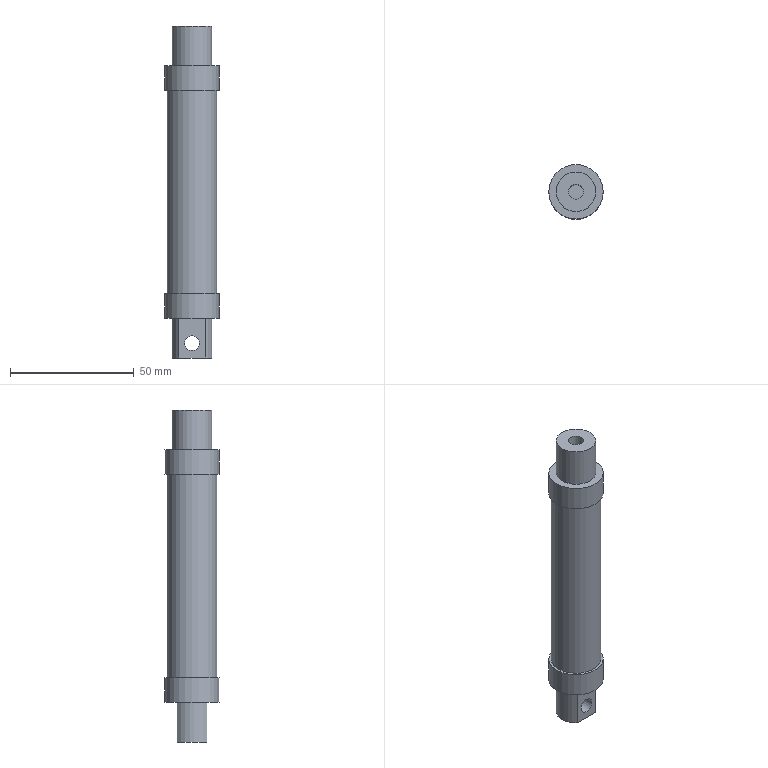Part | NX | features BREP 1, DATUM_CSYS 1 | 1 solid | 17 faces | box 22 x 22 x 134 mm | volume 36167 mm3 | plane 9 | cylinder 8 | commonest cylinder face diameters 16 x3 6 x2 22 x2 20 x1
STEP:
#1=CARTESIAN_POINT('',(11.,0.,92.));
#2=VERTEX_POINT('',#1);
#3=CARTESIAN_POINT('',(0.,0.,92.));
#4=DIRECTION('',(0.,0.,1.));
#5=DIRECTION('',(1.,0.,0.));
#6=AXIS2_PLACEMENT_3D('',#3,#4,#5);
#7=CIRCLE('',#6,11.);
#8=EDGE_CURVE('',#2,#2,#7,.T.);
#9=ORIENTED_EDGE('',*,*,#8,.T.);
#10=EDGE_LOOP('',(#9));
#11=FACE_BOUND('',#10,.T.);
#12=CARTESIAN_POINT('',(8.,0.,92.));
#13=VERTEX_POINT('',#12);
#14=CARTESIAN_POINT('',(0.,0.,92.));
#15=DIRECTION('',(0.,0.,1.));
#16=DIRECTION('',(1.,0.,0.));
#17=AXIS2_PLACEMENT_3D('',#14,#15,#16);
#18=CIRCLE('',#17,8.);
#19=EDGE_CURVE('',#13,#13,#18,.T.);
#20=ORIENTED_EDGE('',*,*,#19,.F.);
#21=EDGE_LOOP('',(#20));
#22=FACE_BOUND('',#21,.T.);
#23=CARTESIAN_POINT('',(0.,0.,92.));
#24=DIRECTION('',(0.,0.,1.));
#25=DIRECTION('',(-1.,0.,0.));
#26=AXIS2_PLACEMENT_3D('',#23,#24,#25);
#27=PLANE('',#26);
#28=ADVANCED_FACE('',(#11,#22),#27,.T.);
#29=CARTESIAN_POINT('',(11.,0.,82.));
#30=VERTEX_POINT('',#29);
#31=CARTESIAN_POINT('',(0.,0.,82.));
#32=DIRECTION('',(0.,0.,1.));
#33=DIRECTION('',(1.,0.,0.));
#34=AXIS2_PLACEMENT_3D('',#31,#32,#33);
#35=CIRCLE('',#34,11.);
#36=EDGE_CURVE('',#30,#30,#35,.T.);
#37=ORIENTED_EDGE('',*,*,#36,.T.);
#38=CARTESIAN_POINT('',(11.,0.,82.));
#39=DIRECTION('',(0.,0.,1.));
#40=VECTOR('',#39,1000.);
#41=LINE('',#38,#40);
#42=EDGE_CURVE('',#30,#2,#41,.T.);
#43=ORIENTED_EDGE('',*,*,#42,.T.);
#44=ORIENTED_EDGE('',*,*,#8,.F.);
#45=ORIENTED_EDGE('',*,*,#42,.F.);
#46=EDGE_LOOP('',(#37,#43,#44,#45));
#47=FACE_BOUND('',#46,.T.);
#48=CARTESIAN_POINT('',(0.,0.,82.));
#49=DIRECTION('',(0.,0.,1.));
#50=DIRECTION('',(-1.,0.,0.));
#51=AXIS2_PLACEMENT_3D('',#48,#49,#50);
#52=CYLINDRICAL_SURFACE('',#51,11.);
#53=ADVANCED_FACE('',(#47),#52,.T.);
#54=ORIENTED_EDGE('',*,*,#36,.F.);
#55=EDGE_LOOP('',(#54));
#56=FACE_BOUND('',#55,.T.);
#57=CARTESIAN_POINT('',(10.,0.,82.));
#58=VERTEX_POINT('',#57);
#59=CARTESIAN_POINT('',(0.,0.,82.));
#60=DIRECTION('',(0.,0.,1.));
#61=DIRECTION('',(1.,0.,0.));
#62=AXIS2_PLACEMENT_3D('',#59,#60,#61);
#63=CIRCLE('',#62,10.);
#64=EDGE_CURVE('',#58,#58,#63,.T.);
#65=ORIENTED_EDGE('',*,*,#64,.T.);
#66=EDGE_LOOP('',(#65));
#67=FACE_BOUND('',#66,.T.);
#68=CARTESIAN_POINT('',(0.,0.,82.));
#69=DIRECTION('',(0.,0.,1.));
#70=DIRECTION('',(-1.,0.,0.));
#71=AXIS2_PLACEMENT_3D('',#68,#69,#70);
#72=PLANE('',#71);
#73=ADVANCED_FACE('',(#56,#67),#72,.F.);
#74=CARTESIAN_POINT('',(10.,0.,0.));
#75=VERTEX_POINT('',#74);
#76=CARTESIAN_POINT('',(0.,0.,0.));
#77=DIRECTION('',(0.,0.,1.));
#78=DIRECTION('',(1.,0.,0.));
#79=AXIS2_PLACEMENT_3D('',#76,#77,#78);
#80=CIRCLE('',#79,10.);
#81=EDGE_CURVE('',#75,#75,#80,.T.);
#82=ORIENTED_EDGE('',*,*,#81,.T.);
#83=CARTESIAN_POINT('',(10.,0.,0.));
#84=DIRECTION('',(0.,0.,1.));
#85=VECTOR('',#84,1000.);
#86=LINE('',#83,#85);
#87=EDGE_CURVE('',#75,#58,#86,.T.);
#88=ORIENTED_EDGE('',*,*,#87,.T.);
#89=ORIENTED_EDGE('',*,*,#64,.F.);
#90=ORIENTED_EDGE('',*,*,#87,.F.);
#91=EDGE_LOOP('',(#82,#88,#89,#90));
#92=FACE_BOUND('',#91,.T.);
#93=CARTESIAN_POINT('',(0.,0.,0.));
#94=DIRECTION('',(0.,0.,1.));
#95=DIRECTION('',(-1.,0.,0.));
#96=AXIS2_PLACEMENT_3D('',#93,#94,#95);
#97=CYLINDRICAL_SURFACE('',#96,10.);
#98=ADVANCED_FACE('',(#92),#97,.T.);
#99=CARTESIAN_POINT('',(11.,0.,0.));
#100=VERTEX_POINT('',#99);
#101=CARTESIAN_POINT('',(0.,0.,0.));
#102=DIRECTION('',(0.,0.,-1.));
#103=DIRECTION('',(1.,0.,0.));
#104=AXIS2_PLACEMENT_3D('',#101,#102,#103);
#105=CIRCLE('',#104,11.);
#106=EDGE_CURVE('',#100,#100,#105,.T.);
#107=ORIENTED_EDGE('',*,*,#106,.F.);
#108=EDGE_LOOP('',(#107));
#109=FACE_BOUND('',#108,.T.);
#110=ORIENTED_EDGE('',*,*,#81,.F.);
#111=EDGE_LOOP('',(#110));
#112=FACE_BOUND('',#111,.T.);
#113=CARTESIAN_POINT('',(0.,0.,0.));
#114=DIRECTION('',(0.,0.,-1.));
#115=DIRECTION('',(-1.,0.,0.));
#116=AXIS2_PLACEMENT_3D('',#113,#114,#115);
#117=PLANE('',#116);
#118=ADVANCED_FACE('',(#109,#112),#117,.F.);
#119=ORIENTED_EDGE('',*,*,#106,.T.);
#120=CARTESIAN_POINT('',(11.,0.,-10.));
#121=VERTEX_POINT('',#120);
#122=CARTESIAN_POINT('',(11.,0.,0.));
#123=DIRECTION('',(0.,0.,-1.));
#124=VECTOR('',#123,1000.);
#125=LINE('',#122,#124);
#126=EDGE_CURVE('',#100,#121,#125,.T.);
#127=ORIENTED_EDGE('',*,*,#126,.T.);
#128=CARTESIAN_POINT('',(0.,0.,-10.));
#129=DIRECTION('',(0.,0.,-1.));
#130=DIRECTION('',(1.,0.,0.));
#131=AXIS2_PLACEMENT_3D('',#128,#129,#130);
#132=CIRCLE('',#131,11.);
#133=EDGE_CURVE('',#121,#121,#132,.T.);
#134=ORIENTED_EDGE('',*,*,#133,.F.);
#135=ORIENTED_EDGE('',*,*,#126,.F.);
#136=EDGE_LOOP('',(#119,#127,#134,#135));
#137=FACE_BOUND('',#136,.T.);
#138=CARTESIAN_POINT('',(0.,0.,0.));
#139=DIRECTION('',(0.,0.,-1.));
#140=DIRECTION('',(-1.,0.,0.));
#141=AXIS2_PLACEMENT_3D('',#138,#139,#140);
#142=CYLINDRICAL_SURFACE('',#141,11.);
#143=ADVANCED_FACE('',(#137),#142,.T.);
#144=ORIENTED_EDGE('',*,*,#133,.T.);
#145=EDGE_LOOP('',(#144));
#146=FACE_BOUND('',#145,.T.);
#147=CARTESIAN_POINT('',(5.292,-6.,-10.));
#148=VERTEX_POINT('',#147);
#149=CARTESIAN_POINT('',(5.292,6.,-10.));
#150=VERTEX_POINT('',#149);
#151=CARTESIAN_POINT('',(0.,0.,-10.));
#152=DIRECTION('',(0.,0.,1.));
#153=DIRECTION('',(0.6614,-0.75,0.));
#154=AXIS2_PLACEMENT_3D('',#151,#152,#153);
#155=CIRCLE('',#154,8.);
#156=EDGE_CURVE('',#148,#150,#155,.T.);
#157=ORIENTED_EDGE('',*,*,#156,.T.);
#158=CARTESIAN_POINT('',(-5.292,6.,-10.));
#159=VERTEX_POINT('',#158);
#160=CARTESIAN_POINT('',(5.292,6.,-10.));
#161=DIRECTION('',(-1.,0.,0.));
#162=VECTOR('',#161,1000.);
#163=LINE('',#160,#162);
#164=EDGE_CURVE('',#150,#159,#163,.T.);
#165=ORIENTED_EDGE('',*,*,#164,.T.);
#166=CARTESIAN_POINT('',(-5.292,-6.,-10.));
#167=VERTEX_POINT('',#166);
#168=CARTESIAN_POINT('',(0.,0.,-10.));
#169=DIRECTION('',(0.,0.,-1.));
#170=DIRECTION('',(-0.6614,-0.75,0.));
#171=AXIS2_PLACEMENT_3D('',#168,#169,#170);
#172=CIRCLE('',#171,8.);
#173=EDGE_CURVE('',#167,#159,#172,.T.);
#174=ORIENTED_EDGE('',*,*,#173,.F.);
#175=CARTESIAN_POINT('',(-5.292,-6.,-10.));
#176=DIRECTION('',(1.,0.,0.));
#177=VECTOR('',#176,1000.);
#178=LINE('',#175,#177);
#179=EDGE_CURVE('',#167,#148,#178,.T.);
#180=ORIENTED_EDGE('',*,*,#179,.T.);
#181=EDGE_LOOP('',(#157,#165,#174,#180));
#182=FACE_BOUND('',#181,.T.);
#183=CARTESIAN_POINT('',(0.,-19.238,-10.));
#184=DIRECTION('',(0.,0.,-1.));
#185=DIRECTION('',(-1.,0.,0.));
#186=AXIS2_PLACEMENT_3D('',#183,#184,#185);
#187=PLANE('',#186);
#188=ADVANCED_FACE('',(#146,#182),#187,.T.);
#189=CARTESIAN_POINT('',(-5.292,-6.,-26.));
#190=VERTEX_POINT('',#189);
#191=CARTESIAN_POINT('',(5.292,-6.,-26.));
#192=VERTEX_POINT('',#191);
#193=CARTESIAN_POINT('',(-5.292,-6.,-26.));
#194=DIRECTION('',(1.,0.,0.));
#195=VECTOR('',#194,1000.);
#196=LINE('',#193,#195);
#197=EDGE_CURVE('',#190,#192,#196,.T.);
#198=ORIENTED_EDGE('',*,*,#197,.F.);
#199=CARTESIAN_POINT('',(-5.292,6.,-26.));
#200=VERTEX_POINT('',#199);
#201=CARTESIAN_POINT('',(0.,0.,-26.));
#202=DIRECTION('',(0.,0.,-1.));
#203=DIRECTION('',(-0.6614,-0.75,0.));
#204=AXIS2_PLACEMENT_3D('',#201,#202,#203);
#205=CIRCLE('',#204,8.);
#206=EDGE_CURVE('',#190,#200,#205,.T.);
#207=ORIENTED_EDGE('',*,*,#206,.T.);
#208=CARTESIAN_POINT('',(5.292,6.,-26.));
#209=VERTEX_POINT('',#208);
#210=CARTESIAN_POINT('',(5.292,6.,-26.));
#211=DIRECTION('',(-1.,0.,0.));
#212=VECTOR('',#211,1000.);
#213=LINE('',#210,#212);
#214=EDGE_CURVE('',#209,#200,#213,.T.);
#215=ORIENTED_EDGE('',*,*,#214,.F.);
#216=CARTESIAN_POINT('',(0.,0.,-26.));
#217=DIRECTION('',(0.,0.,1.));
#218=DIRECTION('',(0.6614,-0.75,0.));
#219=AXIS2_PLACEMENT_3D('',#216,#217,#218);
#220=CIRCLE('',#219,8.);
#221=EDGE_CURVE('',#192,#209,#220,.T.);
#222=ORIENTED_EDGE('',*,*,#221,.F.);
#223=EDGE_LOOP('',(#198,#207,#215,#222));
#224=FACE_BOUND('',#223,.T.);
#225=CARTESIAN_POINT('',(0.,0.,-26.));
#226=DIRECTION('',(0.,0.,-1.));
#227=DIRECTION('',(-1.,0.,0.));
#228=AXIS2_PLACEMENT_3D('',#225,#226,#227);
#229=PLANE('',#228);
#230=ADVANCED_FACE('',(#224),#229,.T.);
#231=CARTESIAN_POINT('',(5.292,6.,-10.));
#232=DIRECTION('',(0.,0.,-1.));
#233=VECTOR('',#232,1000.);
#234=LINE('',#231,#233);
#235=EDGE_CURVE('',#150,#209,#234,.T.);
#236=ORIENTED_EDGE('',*,*,#235,.F.);
#237=ORIENTED_EDGE('',*,*,#156,.F.);
#238=CARTESIAN_POINT('',(5.292,-6.,-26.));
#239=DIRECTION('',(0.,0.,1.));
#240=VECTOR('',#239,1000.);
#241=LINE('',#238,#240);
#242=EDGE_CURVE('',#192,#148,#241,.T.);
#243=ORIENTED_EDGE('',*,*,#242,.F.);
#244=ORIENTED_EDGE('',*,*,#221,.T.);
#245=EDGE_LOOP('',(#236,#237,#243,#244));
#246=FACE_BOUND('',#245,.T.);
#247=CARTESIAN_POINT('',(0.,0.,-10.));
#248=DIRECTION('',(0.,0.,-1.));
#249=DIRECTION('',(-0.6614,-0.75,0.));
#250=AXIS2_PLACEMENT_3D('',#247,#248,#249);
#251=CYLINDRICAL_SURFACE('',#250,8.);
#252=ADVANCED_FACE('',(#246),#251,.T.);
#253=ORIENTED_EDGE('',*,*,#206,.F.);
#254=CARTESIAN_POINT('',(-5.292,-6.,-10.));
#255=DIRECTION('',(0.,0.,-1.));
#256=VECTOR('',#255,1000.);
#257=LINE('',#254,#256);
#258=EDGE_CURVE('',#167,#190,#257,.T.);
#259=ORIENTED_EDGE('',*,*,#258,.F.);
#260=ORIENTED_EDGE('',*,*,#173,.T.);
#261=CARTESIAN_POINT('',(-5.292,6.,-26.));
#262=DIRECTION('',(0.,0.,1.));
#263=VECTOR('',#262,1000.);
#264=LINE('',#261,#263);
#265=EDGE_CURVE('',#200,#159,#264,.T.);
#266=ORIENTED_EDGE('',*,*,#265,.F.);
#267=EDGE_LOOP('',(#253,#259,#260,#266));
#268=FACE_BOUND('',#267,.T.);
#269=CARTESIAN_POINT('',(0.,0.,-10.));
#270=DIRECTION('',(0.,0.,-1.));
#271=DIRECTION('',(-1.,0.,0.));
#272=AXIS2_PLACEMENT_3D('',#269,#270,#271);
#273=CYLINDRICAL_SURFACE('',#272,8.);
#274=ADVANCED_FACE('',(#268),#273,.T.);
#275=ORIENTED_EDGE('',*,*,#197,.T.);
#276=ORIENTED_EDGE('',*,*,#242,.T.);
#277=ORIENTED_EDGE('',*,*,#179,.F.);
#278=ORIENTED_EDGE('',*,*,#258,.T.);
#279=EDGE_LOOP('',(#275,#276,#277,#278));
#280=FACE_BOUND('',#279,.T.);
#281=CARTESIAN_POINT('',(3.,-6.,-20.));
#282=VERTEX_POINT('',#281);
#283=CARTESIAN_POINT('',(0.,-6.,-20.));
#284=DIRECTION('',(0.,1.,0.));
#285=DIRECTION('',(1.,0.,0.));
#286=AXIS2_PLACEMENT_3D('',#283,#284,#285);
#287=CIRCLE('',#286,3.);
#288=EDGE_CURVE('',#282,#282,#287,.T.);
#289=ORIENTED_EDGE('',*,*,#288,.T.);
#290=EDGE_LOOP('',(#289));
#291=FACE_BOUND('',#290,.T.);
#292=CARTESIAN_POINT('',(0.,-6.,-18.));
#293=DIRECTION('',(0.,-1.,0.));
#294=DIRECTION('',(-1.,0.,0.));
#295=AXIS2_PLACEMENT_3D('',#292,#293,#294);
#296=PLANE('',#295);
#297=ADVANCED_FACE('',(#280,#291),#296,.T.);
#298=ORIENTED_EDGE('',*,*,#214,.T.);
#299=ORIENTED_EDGE('',*,*,#265,.T.);
#300=ORIENTED_EDGE('',*,*,#164,.F.);
#301=ORIENTED_EDGE('',*,*,#235,.T.);
#302=EDGE_LOOP('',(#298,#299,#300,#301));
#303=FACE_BOUND('',#302,.T.);
#304=CARTESIAN_POINT('',(3.,6.,-20.));
#305=VERTEX_POINT('',#304);
#306=CARTESIAN_POINT('',(0.,6.,-20.));
#307=DIRECTION('',(0.,1.,0.));
#308=DIRECTION('',(1.,0.,0.));
#309=AXIS2_PLACEMENT_3D('',#306,#307,#308);
#310=CIRCLE('',#309,3.);
#311=EDGE_CURVE('',#305,#305,#310,.T.);
#312=ORIENTED_EDGE('',*,*,#311,.F.);
#313=EDGE_LOOP('',(#312));
#314=FACE_BOUND('',#313,.T.);
#315=CARTESIAN_POINT('',(0.,6.,-18.));
#316=DIRECTION('',(0.,1.,0.));
#317=DIRECTION('',(1.,0.,0.));
#318=AXIS2_PLACEMENT_3D('',#315,#316,#317);
#319=PLANE('',#318);
#320=ADVANCED_FACE('',(#303,#314),#319,.T.);
#321=CARTESIAN_POINT('',(3.,-6.,-20.));
#322=DIRECTION('',(0.,1.,0.));
#323=VECTOR('',#322,1000.);
#324=LINE('',#321,#323);
#325=EDGE_CURVE('',#282,#305,#324,.T.);
#326=ORIENTED_EDGE('',*,*,#325,.T.);
#327=ORIENTED_EDGE('',*,*,#311,.T.);
#328=ORIENTED_EDGE('',*,*,#325,.F.);
#329=ORIENTED_EDGE('',*,*,#288,.F.);
#330=EDGE_LOOP('',(#326,#327,#328,#329));
#331=FACE_BOUND('',#330,.T.);
#332=CARTESIAN_POINT('',(0.,-6.,-20.));
#333=DIRECTION('',(0.,1.,0.));
#334=DIRECTION('',(-1.,0.,0.));
#335=AXIS2_PLACEMENT_3D('',#332,#333,#334);
#336=CYLINDRICAL_SURFACE('',#335,3.);
#337=ADVANCED_FACE('',(#331),#336,.F.);
#338=ORIENTED_EDGE('',*,*,#19,.T.);
#339=CARTESIAN_POINT('',(8.,0.,108.));
#340=VERTEX_POINT('',#339);
#341=CARTESIAN_POINT('',(8.,0.,92.));
#342=DIRECTION('',(0.,0.,1.));
#343=VECTOR('',#342,1000.);
#344=LINE('',#341,#343);
#345=EDGE_CURVE('',#13,#340,#344,.T.);
#346=ORIENTED_EDGE('',*,*,#345,.T.);
#347=CARTESIAN_POINT('',(0.,0.,108.));
#348=DIRECTION('',(0.,0.,1.));
#349=DIRECTION('',(1.,0.,0.));
#350=AXIS2_PLACEMENT_3D('',#347,#348,#349);
#351=CIRCLE('',#350,8.);
#352=EDGE_CURVE('',#340,#340,#351,.T.);
#353=ORIENTED_EDGE('',*,*,#352,.F.);
#354=ORIENTED_EDGE('',*,*,#345,.F.);
#355=EDGE_LOOP('',(#338,#346,#353,#354));
#356=FACE_BOUND('',#355,.T.);
#357=CARTESIAN_POINT('',(0.,0.,92.));
#358=DIRECTION('',(0.,0.,1.));
#359=DIRECTION('',(-1.,0.,0.));
#360=AXIS2_PLACEMENT_3D('',#357,#358,#359);
#361=CYLINDRICAL_SURFACE('',#360,8.);
#362=ADVANCED_FACE('',(#356),#361,.T.);
#363=ORIENTED_EDGE('',*,*,#352,.T.);
#364=EDGE_LOOP('',(#363));
#365=FACE_BOUND('',#364,.T.);
#366=CARTESIAN_POINT('',(3.,0.,108.));
#367=VERTEX_POINT('',#366);
#368=CARTESIAN_POINT('',(0.,0.,108.));
#369=DIRECTION('',(0.,0.,-1.));
#370=DIRECTION('',(1.,0.,0.));
#371=AXIS2_PLACEMENT_3D('',#368,#369,#370);
#372=CIRCLE('',#371,3.);
#373=EDGE_CURVE('',#367,#367,#372,.T.);
#374=ORIENTED_EDGE('',*,*,#373,.T.);
#375=EDGE_LOOP('',(#374));
#376=FACE_BOUND('',#375,.T.);
#377=CARTESIAN_POINT('',(0.,0.,108.));
#378=DIRECTION('',(0.,0.,1.));
#379=DIRECTION('',(-1.,0.,0.));
#380=AXIS2_PLACEMENT_3D('',#377,#378,#379);
#381=PLANE('',#380);
#382=ADVANCED_FACE('',(#365,#376),#381,.T.);
#383=CARTESIAN_POINT('',(3.,0.,8.));
#384=VERTEX_POINT('',#383);
#385=CARTESIAN_POINT('',(3.,0.,108.));
#386=DIRECTION('',(0.,0.,-1.));
#387=VECTOR('',#386,1000.);
#388=LINE('',#385,#387);
#389=EDGE_CURVE('',#367,#384,#388,.T.);
#390=ORIENTED_EDGE('',*,*,#389,.T.);
#391=CARTESIAN_POINT('',(0.,0.,8.));
#392=DIRECTION('',(0.,0.,-1.));
#393=DIRECTION('',(1.,0.,0.));
#394=AXIS2_PLACEMENT_3D('',#391,#392,#393);
#395=CIRCLE('',#394,3.);
#396=EDGE_CURVE('',#384,#384,#395,.T.);
#397=ORIENTED_EDGE('',*,*,#396,.T.);
#398=ORIENTED_EDGE('',*,*,#389,.F.);
#399=ORIENTED_EDGE('',*,*,#373,.F.);
#400=EDGE_LOOP('',(#390,#397,#398,#399));
#401=FACE_BOUND('',#400,.T.);
#402=CARTESIAN_POINT('',(0.,0.,108.));
#403=DIRECTION('',(0.,0.,-1.));
#404=DIRECTION('',(-1.,0.,0.));
#405=AXIS2_PLACEMENT_3D('',#402,#403,#404);
#406=CYLINDRICAL_SURFACE('',#405,3.);
#407=ADVANCED_FACE('',(#401),#406,.F.);
#408=ORIENTED_EDGE('',*,*,#396,.F.);
#409=EDGE_LOOP('',(#408));
#410=FACE_BOUND('',#409,.T.);
#411=CARTESIAN_POINT('',(0.,0.,8.));
#412=DIRECTION('',(0.,0.,-1.));
#413=DIRECTION('',(-1.,0.,0.));
#414=AXIS2_PLACEMENT_3D('',#411,#412,#413);
#415=PLANE('',#414);
#416=ADVANCED_FACE('',(#410),#415,.F.);
#417=CLOSED_SHELL('',(#28,#53,#73,#98,#118,#143,#188,#230,#252,#274,#297,#320,#337,#362,#382,#407,#416));
#418=MANIFOLD_SOLID_BREP('',#417);
#419=(LENGTH_UNIT()NAMED_UNIT(*)SI_UNIT(.MILLI.,.METRE.));
#420=UNCERTAINTY_MEASURE_WITH_UNIT(LENGTH_MEASURE(0.00001),#419,'','');
#421=(NAMED_UNIT(*)PLANE_ANGLE_UNIT()SI_UNIT($,.RADIAN.));
#422=(NAMED_UNIT(*)SI_UNIT($,.STERADIAN.)SOLID_ANGLE_UNIT());
#423=(GEOMETRIC_REPRESENTATION_CONTEXT(3)GLOBAL_UNCERTAINTY_ASSIGNED_CONTEXT((#420))GLOBAL_UNIT_ASSIGNED_CONTEXT((#419,#421,#422))REPRESENTATION_CONTEXT('',''));
#424=ADVANCED_BREP_SHAPE_REPRESENTATION('',(#418),#423);